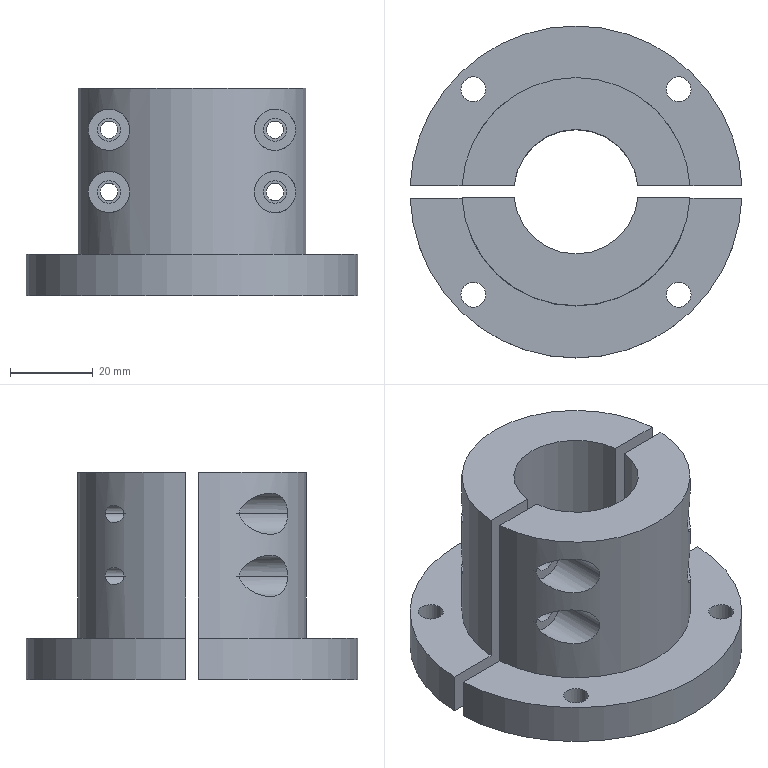Part | 2 solids | 52 faces | box 79.944 x 80 x 50 mm | volume 99773 mm3 | cylinder 38 | plane 14 | commonest cylinder face diameters 4.2 x8 5.5 x8 6 x8 10 x8 30 x2 55 x2